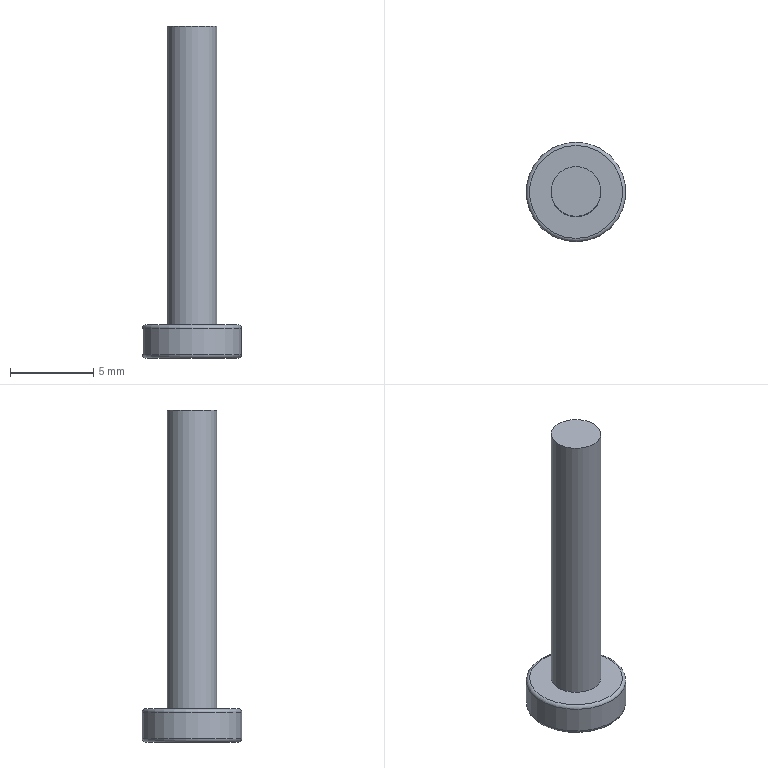Part | STEP file | 1-16.4 | 1 solid | 8 faces | box 6 x 6 x 20 mm | volume 175.087 mm3 | plane 3 | cylinder 2 | torus 2 | cone 1 | commonest cylinder face diameters 3 x1 6 x1
STEP:
#1=CARTESIAN_POINT('',(0.,0.,0.));
#2=DIRECTION('',(0.,0.,1.));
#3=DIRECTION('',(1.,0.,0.));
#4=AXIS2_PLACEMENT_3D('',#1,#2,#3);
#5=CARTESIAN_POINT('',(0.,1.5,0.));
#6=VERTEX_POINT('',#5);
#7=CARTESIAN_POINT('',(0.,0.,0.));
#8=DIRECTION('',(0.,0.,1.));
#9=DIRECTION('',(0.,1.,0.));
#10=AXIS2_PLACEMENT_3D('',#7,#8,#9);
#11=CIRCLE('',#10,1.5);
#12=CARTESIAN_POINT('',(0.,0.,0.));
#13=DIRECTION('',(0.,0.,1.));
#14=DIRECTION('',(0.,1.,0.));
#15=AXIS2_PLACEMENT_3D('',#12,#13,#14);
#16=CYLINDRICAL_SURFACE('',#15,1.5);
#17=CARTESIAN_POINT('',(0.,0.));
#18=DIRECTION('',(1.,0.));
#19=VECTOR('',#18,1.);
#20=LINE('',#17,#19);
#21=(GEOMETRIC_REPRESENTATION_CONTEXT(2)PARAMETRIC_REPRESENTATION_CONTEXT()REPRESENTATION_CONTEXT('',''));
#22=DEFINITIONAL_REPRESENTATION('',(#20),#21);
#23=PCURVE('',#16,#22);
#24=CARTESIAN_POINT('',(0.,-0.8038,0.));
#25=DIRECTION('',(0.,0.,1.));
#26=DIRECTION('',(1.,0.,0.));
#27=AXIS2_PLACEMENT_3D('',#24,#25,#26);
#28=PLANE('',#27);
#29=CARTESIAN_POINT('',(0.,0.8038));
#30=DIRECTION('',(0.,1.));
#31=AXIS2_PLACEMENT_2D('',#29,#30);
#32=CIRCLE('',#31,1.5);
#33=(GEOMETRIC_REPRESENTATION_CONTEXT(2)PARAMETRIC_REPRESENTATION_CONTEXT()REPRESENTATION_CONTEXT('',''));
#34=DEFINITIONAL_REPRESENTATION('',(#32),#33);
#35=PCURVE('',#28,#34);
#36=SURFACE_CURVE('',#11,(#23,#35),.PCURVE_S1.);
#37=EDGE_CURVE('',#6,#6,#36,.T.);
#38=ORIENTED_EDGE('',*,*,#37,.T.);
#39=CARTESIAN_POINT('',(0.,1.5,18.));
#40=VERTEX_POINT('',#39);
#41=CARTESIAN_POINT('',(0.,1.5,0.));
#42=DIRECTION('',(0.,0.,1.));
#43=VECTOR('',#42,1.);
#44=LINE('',#41,#43);
#45=CARTESIAN_POINT('',(6.283,0.));
#46=DIRECTION('',(0.,1.));
#47=VECTOR('',#46,1.);
#48=LINE('',#45,#47);
#49=(GEOMETRIC_REPRESENTATION_CONTEXT(2)PARAMETRIC_REPRESENTATION_CONTEXT()REPRESENTATION_CONTEXT('',''));
#50=DEFINITIONAL_REPRESENTATION('',(#48),#49);
#51=PCURVE('',#16,#50);
#52=CARTESIAN_POINT('',(0.,0.));
#53=DIRECTION('',(0.,1.));
#54=VECTOR('',#53,1.);
#55=LINE('',#52,#54);
#56=(GEOMETRIC_REPRESENTATION_CONTEXT(2)PARAMETRIC_REPRESENTATION_CONTEXT()REPRESENTATION_CONTEXT('',''));
#57=DEFINITIONAL_REPRESENTATION('',(#55),#56);
#58=PCURVE('',#16,#57);
#59=SEAM_CURVE('',#44,(#51,#58),.PCURVE_S1.);
#60=EDGE_CURVE('',#6,#40,#59,.T.);
#61=ORIENTED_EDGE('',*,*,#60,.T.);
#62=CARTESIAN_POINT('',(0.,0.,18.));
#63=DIRECTION('',(0.,0.,1.));
#64=DIRECTION('',(0.,1.,0.));
#65=AXIS2_PLACEMENT_3D('',#62,#63,#64);
#66=CIRCLE('',#65,1.5);
#67=CARTESIAN_POINT('',(0.,18.));
#68=DIRECTION('',(1.,0.));
#69=VECTOR('',#68,1.);
#70=LINE('',#67,#69);
#71=(GEOMETRIC_REPRESENTATION_CONTEXT(2)PARAMETRIC_REPRESENTATION_CONTEXT()REPRESENTATION_CONTEXT('',''));
#72=DEFINITIONAL_REPRESENTATION('',(#70),#71);
#73=PCURVE('',#16,#72);
#74=CARTESIAN_POINT('',(0.,-0.4019,18.));
#75=DIRECTION('',(0.,0.,1.));
#76=DIRECTION('',(1.,0.,0.));
#77=AXIS2_PLACEMENT_3D('',#74,#75,#76);
#78=PLANE('',#77);
#79=CARTESIAN_POINT('',(0.,0.4019));
#80=DIRECTION('',(0.,1.));
#81=AXIS2_PLACEMENT_2D('',#79,#80);
#82=CIRCLE('',#81,1.5);
#83=(GEOMETRIC_REPRESENTATION_CONTEXT(2)PARAMETRIC_REPRESENTATION_CONTEXT()REPRESENTATION_CONTEXT('',''));
#84=DEFINITIONAL_REPRESENTATION('',(#82),#83);
#85=PCURVE('',#78,#84);
#86=SURFACE_CURVE('',#66,(#73,#85),.PCURVE_S1.);
#87=EDGE_CURVE('',#40,#40,#86,.T.);
#88=ORIENTED_EDGE('',*,*,#87,.F.);
#89=ORIENTED_EDGE('',*,*,#60,.F.);
#90=EDGE_LOOP('',(#38,#61,#88,#89));
#91=FACE_BOUND('',#90,.T.);
#92=ADVANCED_FACE('',(#91),#16,.T.);
#93=ORIENTED_EDGE('',*,*,#87,.T.);
#94=EDGE_LOOP('',(#93));
#95=FACE_BOUND('',#94,.T.);
#96=ADVANCED_FACE('',(#95),#78,.T.);
#97=CARTESIAN_POINT('',(0.,3.,-0.2));
#98=VERTEX_POINT('',#97);
#99=CARTESIAN_POINT('',(0.,0.,-0.2));
#100=DIRECTION('',(0.,0.,1.));
#101=DIRECTION('',(0.,1.,0.));
#102=AXIS2_PLACEMENT_3D('',#99,#100,#101);
#103=CIRCLE('',#102,3.);
#104=CARTESIAN_POINT('',(0.,0.,0.));
#105=DIRECTION('',(0.,0.,-1.));
#106=DIRECTION('',(0.,1.,0.));
#107=AXIS2_PLACEMENT_3D('',#104,#105,#106);
#108=CYLINDRICAL_SURFACE('',#107,3.);
#109=CARTESIAN_POINT('',(6.283,0.2));
#110=DIRECTION('',(-1.,0.));
#111=VECTOR('',#110,1.);
#112=LINE('',#109,#111);
#113=(GEOMETRIC_REPRESENTATION_CONTEXT(2)PARAMETRIC_REPRESENTATION_CONTEXT()REPRESENTATION_CONTEXT('',''));
#114=DEFINITIONAL_REPRESENTATION('',(#112),#113);
#115=PCURVE('',#108,#114);
#116=CARTESIAN_POINT('',(0.,0.,-0.2));
#117=DIRECTION('',(0.,0.,-1.));
#118=DIRECTION('',(0.,1.,0.));
#119=AXIS2_PLACEMENT_3D('',#116,#117,#118);
#120=TOROIDAL_SURFACE('',#119,2.8,0.2);
#121=CARTESIAN_POINT('',(6.283,6.283));
#122=DIRECTION('',(-1.,0.));
#123=VECTOR('',#122,1.);
#124=LINE('',#121,#123);
#125=(GEOMETRIC_REPRESENTATION_CONTEXT(2)PARAMETRIC_REPRESENTATION_CONTEXT()REPRESENTATION_CONTEXT('',''));
#126=DEFINITIONAL_REPRESENTATION('',(#124),#125);
#127=PCURVE('',#120,#126);
#128=SURFACE_CURVE('',#103,(#115,#127),.PCURVE_S1.);
#129=EDGE_CURVE('',#98,#98,#128,.T.);
#130=ORIENTED_EDGE('',*,*,#129,.F.);
#131=CARTESIAN_POINT('',(0.,3.,-1.8));
#132=VERTEX_POINT('',#131);
#133=CARTESIAN_POINT('',(0.,3.,-0.2));
#134=DIRECTION('',(0.,0.,-1.));
#135=VECTOR('',#134,1.);
#136=LINE('',#133,#135);
#137=CARTESIAN_POINT('',(6.283,0.2));
#138=DIRECTION('',(0.,1.));
#139=VECTOR('',#138,1.);
#140=LINE('',#137,#139);
#141=(GEOMETRIC_REPRESENTATION_CONTEXT(2)PARAMETRIC_REPRESENTATION_CONTEXT()REPRESENTATION_CONTEXT('',''));
#142=DEFINITIONAL_REPRESENTATION('',(#140),#141);
#143=PCURVE('',#108,#142);
#144=CARTESIAN_POINT('',(0.,0.2));
#145=DIRECTION('',(0.,1.));
#146=VECTOR('',#145,1.);
#147=LINE('',#144,#146);
#148=(GEOMETRIC_REPRESENTATION_CONTEXT(2)PARAMETRIC_REPRESENTATION_CONTEXT()REPRESENTATION_CONTEXT('',''));
#149=DEFINITIONAL_REPRESENTATION('',(#147),#148);
#150=PCURVE('',#108,#149);
#151=SEAM_CURVE('',#136,(#143,#150),.PCURVE_S1.);
#152=EDGE_CURVE('',#98,#132,#151,.T.);
#153=ORIENTED_EDGE('',*,*,#152,.T.);
#154=CARTESIAN_POINT('',(0.,0.,-1.8));
#155=DIRECTION('',(0.,0.,1.));
#156=DIRECTION('',(0.,1.,0.));
#157=AXIS2_PLACEMENT_3D('',#154,#155,#156);
#158=CIRCLE('',#157,3.);
#159=CARTESIAN_POINT('',(6.283,1.8));
#160=DIRECTION('',(-1.,0.));
#161=VECTOR('',#160,1.);
#162=LINE('',#159,#161);
#163=(GEOMETRIC_REPRESENTATION_CONTEXT(2)PARAMETRIC_REPRESENTATION_CONTEXT()REPRESENTATION_CONTEXT('',''));
#164=DEFINITIONAL_REPRESENTATION('',(#162),#163);
#165=PCURVE('',#108,#164);
#166=CARTESIAN_POINT('',(0.,0.,-1.8));
#167=DIRECTION('',(0.,0.,-1.));
#168=DIRECTION('',(0.,1.,0.));
#169=AXIS2_PLACEMENT_3D('',#166,#167,#168);
#170=TOROIDAL_SURFACE('',#169,2.8,0.2);
#171=CARTESIAN_POINT('',(6.283,0.));
#172=DIRECTION('',(-1.,0.));
#173=VECTOR('',#172,1.);
#174=LINE('',#171,#173);
#175=(GEOMETRIC_REPRESENTATION_CONTEXT(2)PARAMETRIC_REPRESENTATION_CONTEXT()REPRESENTATION_CONTEXT('',''));
#176=DEFINITIONAL_REPRESENTATION('',(#174),#175);
#177=PCURVE('',#170,#176);
#178=SURFACE_CURVE('',#158,(#165,#177),.PCURVE_S1.);
#179=EDGE_CURVE('',#132,#132,#178,.T.);
#180=ORIENTED_EDGE('',*,*,#179,.T.);
#181=ORIENTED_EDGE('',*,*,#152,.F.);
#182=EDGE_LOOP('',(#130,#153,#180,#181));
#183=FACE_BOUND('',#182,.T.);
#184=ADVANCED_FACE('',(#183),#108,.T.);
#185=CARTESIAN_POINT('',(0.,2.8,0.));
#186=VERTEX_POINT('',#185);
#187=CARTESIAN_POINT('',(0.,0.,0.));
#188=DIRECTION('',(0.,0.,1.));
#189=DIRECTION('',(0.,1.,0.));
#190=AXIS2_PLACEMENT_3D('',#187,#188,#189);
#191=CIRCLE('',#190,2.8);
#192=CARTESIAN_POINT('',(0.,0.8038));
#193=DIRECTION('',(0.,1.));
#194=AXIS2_PLACEMENT_2D('',#192,#193);
#195=CIRCLE('',#194,2.8);
#196=(GEOMETRIC_REPRESENTATION_CONTEXT(2)PARAMETRIC_REPRESENTATION_CONTEXT()REPRESENTATION_CONTEXT('',''));
#197=DEFINITIONAL_REPRESENTATION('',(#195),#196);
#198=PCURVE('',#28,#197);
#199=CARTESIAN_POINT('',(6.283,4.712));
#200=DIRECTION('',(-1.,0.));
#201=VECTOR('',#200,1.);
#202=LINE('',#199,#201);
#203=(GEOMETRIC_REPRESENTATION_CONTEXT(2)PARAMETRIC_REPRESENTATION_CONTEXT()REPRESENTATION_CONTEXT('',''));
#204=DEFINITIONAL_REPRESENTATION('',(#202),#203);
#205=PCURVE('',#120,#204);
#206=SURFACE_CURVE('',#191,(#198,#205),.PCURVE_S1.);
#207=EDGE_CURVE('',#186,#186,#206,.T.);
#208=ORIENTED_EDGE('',*,*,#207,.T.);
#209=EDGE_LOOP('',(#208));
#210=FACE_BOUND('',#209,.T.);
#211=ORIENTED_EDGE('',*,*,#37,.F.);
#212=EDGE_LOOP('',(#211));
#213=FACE_BOUND('',#212,.T.);
#214=ADVANCED_FACE('',(#210,#213),#28,.T.);
#215=ORIENTED_EDGE('',*,*,#207,.F.);
#216=CARTESIAN_POINT('',(0.,2.8,-0.2));
#217=DIRECTION('',(-1.,0.,0.));
#218=DIRECTION('',(0.,0.,1.));
#219=AXIS2_PLACEMENT_3D('',#216,#217,#218);
#220=CIRCLE('',#219,0.2);
#221=CARTESIAN_POINT('',(6.283,4.712));
#222=DIRECTION('',(0.,1.));
#223=VECTOR('',#222,1.);
#224=LINE('',#221,#223);
#225=(GEOMETRIC_REPRESENTATION_CONTEXT(2)PARAMETRIC_REPRESENTATION_CONTEXT()REPRESENTATION_CONTEXT('',''));
#226=DEFINITIONAL_REPRESENTATION('',(#224),#225);
#227=PCURVE('',#120,#226);
#228=CARTESIAN_POINT('',(0.,4.712));
#229=DIRECTION('',(0.,1.));
#230=VECTOR('',#229,1.);
#231=LINE('',#228,#230);
#232=(GEOMETRIC_REPRESENTATION_CONTEXT(2)PARAMETRIC_REPRESENTATION_CONTEXT()REPRESENTATION_CONTEXT('',''));
#233=DEFINITIONAL_REPRESENTATION('',(#231),#232);
#234=PCURVE('',#120,#233);
#235=SEAM_CURVE('',#220,(#227,#234),.PCURVE_S1.);
#236=EDGE_CURVE('',#186,#98,#235,.T.);
#237=ORIENTED_EDGE('',*,*,#236,.T.);
#238=ORIENTED_EDGE('',*,*,#129,.T.);
#239=ORIENTED_EDGE('',*,*,#236,.F.);
#240=EDGE_LOOP('',(#215,#237,#238,#239));
#241=FACE_BOUND('',#240,.T.);
#242=ADVANCED_FACE('',(#241),#120,.T.);
#243=CARTESIAN_POINT('',(0.,2.8,-2.));
#244=VERTEX_POINT('',#243);
#245=CARTESIAN_POINT('',(0.,2.8,-1.8));
#246=DIRECTION('',(1.,0.,0.));
#247=DIRECTION('',(0.,0.,-1.));
#248=AXIS2_PLACEMENT_3D('',#245,#246,#247);
#249=CIRCLE('',#248,0.2);
#250=CARTESIAN_POINT('',(0.,1.571));
#251=DIRECTION('',(0.,-1.));
#252=VECTOR('',#251,1.);
#253=LINE('',#250,#252);
#254=(GEOMETRIC_REPRESENTATION_CONTEXT(2)PARAMETRIC_REPRESENTATION_CONTEXT()REPRESENTATION_CONTEXT('',''));
#255=DEFINITIONAL_REPRESENTATION('',(#253),#254);
#256=PCURVE('',#170,#255);
#257=CARTESIAN_POINT('',(6.283,1.571));
#258=DIRECTION('',(0.,-1.));
#259=VECTOR('',#258,1.);
#260=LINE('',#257,#259);
#261=(GEOMETRIC_REPRESENTATION_CONTEXT(2)PARAMETRIC_REPRESENTATION_CONTEXT()REPRESENTATION_CONTEXT('',''));
#262=DEFINITIONAL_REPRESENTATION('',(#260),#261);
#263=PCURVE('',#170,#262);
#264=SEAM_CURVE('',#249,(#256,#263),.PCURVE_S1.);
#265=EDGE_CURVE('',#244,#132,#264,.T.);
#266=ORIENTED_EDGE('',*,*,#265,.T.);
#267=ORIENTED_EDGE('',*,*,#179,.F.);
#268=ORIENTED_EDGE('',*,*,#265,.F.);
#269=CARTESIAN_POINT('',(0.,0.,-2.));
#270=DIRECTION('',(0.,0.,1.));
#271=DIRECTION('',(0.,1.,0.));
#272=AXIS2_PLACEMENT_3D('',#269,#270,#271);
#273=CIRCLE('',#272,2.8);
#274=CARTESIAN_POINT('',(6.283,1.571));
#275=DIRECTION('',(-1.,0.));
#276=VECTOR('',#275,1.);
#277=LINE('',#274,#276);
#278=(GEOMETRIC_REPRESENTATION_CONTEXT(2)PARAMETRIC_REPRESENTATION_CONTEXT()REPRESENTATION_CONTEXT('',''));
#279=DEFINITIONAL_REPRESENTATION('',(#277),#278);
#280=PCURVE('',#170,#279);
#281=CARTESIAN_POINT('',(0.,-0.8038,-2.));
#282=DIRECTION('',(0.,0.,1.));
#283=DIRECTION('',(1.,0.,0.));
#284=AXIS2_PLACEMENT_3D('',#281,#282,#283);
#285=PLANE('',#284);
#286=CARTESIAN_POINT('',(0.,0.8038));
#287=DIRECTION('',(0.,1.));
#288=AXIS2_PLACEMENT_2D('',#286,#287);
#289=CIRCLE('',#288,2.8);
#290=(GEOMETRIC_REPRESENTATION_CONTEXT(2)PARAMETRIC_REPRESENTATION_CONTEXT()REPRESENTATION_CONTEXT('',''));
#291=DEFINITIONAL_REPRESENTATION('',(#289),#290);
#292=PCURVE('',#285,#291);
#293=SURFACE_CURVE('',#273,(#280,#292),.PCURVE_S1.);
#294=EDGE_CURVE('',#244,#244,#293,.T.);
#295=ORIENTED_EDGE('',*,*,#294,.T.);
#296=EDGE_LOOP('',(#266,#267,#268,#295));
#297=FACE_BOUND('',#296,.T.);
#298=ADVANCED_FACE('',(#297),#170,.T.);
#299=ORIENTED_EDGE('',*,*,#294,.T.);
#300=EDGE_LOOP('',(#299));
#301=FACE_BOUND('',#300,.F.);
#302=CARTESIAN_POINT('',(0.,2.,-2.));
#303=VERTEX_POINT('',#302);
#304=CARTESIAN_POINT('',(0.,0.,-2.));
#305=DIRECTION('',(0.,0.,-1.));
#306=DIRECTION('',(0.,1.,0.));
#307=AXIS2_PLACEMENT_3D('',#304,#305,#306);
#308=CIRCLE('',#307,2.);
#309=CARTESIAN_POINT('',(0.,2.804));
#310=CARTESIAN_POINT('',(3.464,2.804));
#311=CARTESIAN_POINT('',(1.732,-0.1962));
#312=CARTESIAN_POINT('',(0.,-3.196));
#313=CARTESIAN_POINT('',(-1.732,-0.1962));
#314=CARTESIAN_POINT('',(-3.464,2.804));
#315=CARTESIAN_POINT('',(0.,2.804));
#316=(BOUNDED_CURVE()B_SPLINE_CURVE(2,(#309,#310,#311,#312,#313,#314,#315),.UNSPECIFIED.,.T.,.F.)B_SPLINE_CURVE_WITH_KNOTS((1,2,2,2,2,1),(-2.094,0.,2.094,4.189,6.283,8.378),.UNSPECIFIED.)CURVE()GEOMETRIC_REPRESENTATION_ITEM()RATIONAL_B_SPLINE_CURVE((1.,0.5,1.,0.5,1.,0.5,1.))REPRESENTATION_ITEM(''));
#317=(GEOMETRIC_REPRESENTATION_CONTEXT(2)PARAMETRIC_REPRESENTATION_CONTEXT()REPRESENTATION_CONTEXT('',''));
#318=DEFINITIONAL_REPRESENTATION('',(#316),#317);
#319=PCURVE('',#285,#318);
#320=CARTESIAN_POINT('',(0.,0.,0.));
#321=DIRECTION('',(0.,0.,-1.));
#322=DIRECTION('',(0.,1.,0.));
#323=AXIS2_PLACEMENT_3D('',#320,#321,#322);
#324=CONICAL_SURFACE('',#323,0.,0.7854);
#325=CARTESIAN_POINT('',(0.,2.));
#326=DIRECTION('',(1.,0.));
#327=VECTOR('',#326,1.);
#328=LINE('',#325,#327);
#329=(GEOMETRIC_REPRESENTATION_CONTEXT(2)PARAMETRIC_REPRESENTATION_CONTEXT()REPRESENTATION_CONTEXT('',''));
#330=DEFINITIONAL_REPRESENTATION('',(#328),#329);
#331=PCURVE('',#324,#330);
#332=SURFACE_CURVE('',#308,(#319,#331),.PCURVE_S1.);
#333=EDGE_CURVE('',#303,#303,#332,.T.);
#334=ORIENTED_EDGE('',*,*,#333,.T.);
#335=EDGE_LOOP('',(#334));
#336=FACE_BOUND('',#335,.F.);
#337=ADVANCED_FACE('',(#301,#336),#285,.F.);
#338=CARTESIAN_POINT('',(0.,0.,0.));
#339=VERTEX_POINT('',#338);
#340=CARTESIAN_POINT('',(0.,2.,-2.));
#341=DIRECTION('',(0.,-0.7071,0.7071));
#342=VECTOR('',#341,1.);
#343=LINE('',#340,#342);
#344=CARTESIAN_POINT('',(0.,2.));
#345=CARTESIAN_POINT('',(0.,1.97));
#346=CARTESIAN_POINT('',(0.,1.909));
#347=CARTESIAN_POINT('',(0.,1.818));
#348=CARTESIAN_POINT('',(0.,1.727));
#349=CARTESIAN_POINT('',(0.,1.636));
#350=CARTESIAN_POINT('',(0.,1.545));
#351=CARTESIAN_POINT('',(0.,1.455));
#352=CARTESIAN_POINT('',(0.,1.364));
#353=CARTESIAN_POINT('',(0.,1.273));
#354=CARTESIAN_POINT('',(0.,1.182));
#355=CARTESIAN_POINT('',(0.,1.091));
#356=CARTESIAN_POINT('',(0.,1.));
#357=CARTESIAN_POINT('',(0.,0.9091));
#358=CARTESIAN_POINT('',(0.,0.8182));
#359=CARTESIAN_POINT('',(0.,0.7273));
#360=CARTESIAN_POINT('',(0.,0.6364));
#361=CARTESIAN_POINT('',(0.,0.5455));
#362=CARTESIAN_POINT('',(0.,0.4545));
#363=CARTESIAN_POINT('',(0.,0.3636));
#364=CARTESIAN_POINT('',(0.,0.2727));
#365=CARTESIAN_POINT('',(0.,0.1818));
#366=CARTESIAN_POINT('',(0.,0.09091));
#367=CARTESIAN_POINT('',(0.,0.0303));
#368=CARTESIAN_POINT('',(0.,0.));
#369=B_SPLINE_CURVE_WITH_KNOTS('',3,(#344,#345,#346,#347,#348,#349,#350,#351,#352,#353,#354,#355,#356,#357,#358,#359,#360,#361,#362,#363,#364,#365,#366,#367,#368),.UNSPECIFIED.,.F.,.F.,(4,1,1,1,1,1,1,1,1,1,1,1,1,1,1,1,1,1,1,1,1,1,4),(0.,0.1286,0.2571,0.3857,0.5143,0.6428,0.7714,0.9,1.029,1.157,1.286,1.414,1.543,1.671,1.8,1.928,2.057,2.186,2.314,2.443,2.571,2.7,2.828),.QUASI_UNIFORM_KNOTS.);
#370=(GEOMETRIC_REPRESENTATION_CONTEXT(2)PARAMETRIC_REPRESENTATION_CONTEXT()REPRESENTATION_CONTEXT('',''));
#371=DEFINITIONAL_REPRESENTATION('',(#369),#370);
#372=PCURVE('',#324,#371);
#373=CARTESIAN_POINT('',(6.283,2.));
#374=CARTESIAN_POINT('',(6.283,1.97));
#375=CARTESIAN_POINT('',(6.283,1.909));
#376=CARTESIAN_POINT('',(6.283,1.818));
#377=CARTESIAN_POINT('',(6.283,1.727));
#378=CARTESIAN_POINT('',(6.283,1.636));
#379=CARTESIAN_POINT('',(6.283,1.545));
#380=CARTESIAN_POINT('',(6.283,1.455));
#381=CARTESIAN_POINT('',(6.283,1.364));
#382=CARTESIAN_POINT('',(6.283,1.273));
#383=CARTESIAN_POINT('',(6.283,1.182));
#384=CARTESIAN_POINT('',(6.283,1.091));
#385=CARTESIAN_POINT('',(6.283,1.));
#386=CARTESIAN_POINT('',(6.283,0.9091));
#387=CARTESIAN_POINT('',(6.283,0.8182));
#388=CARTESIAN_POINT('',(6.283,0.7273));
#389=CARTESIAN_POINT('',(6.283,0.6364));
#390=CARTESIAN_POINT('',(6.283,0.5455));
#391=CARTESIAN_POINT('',(6.283,0.4545));
#392=CARTESIAN_POINT('',(6.283,0.3636));
#393=CARTESIAN_POINT('',(6.283,0.2727));
#394=CARTESIAN_POINT('',(6.283,0.1818));
#395=CARTESIAN_POINT('',(6.283,0.09091));
#396=CARTESIAN_POINT('',(6.283,0.0303));
#397=CARTESIAN_POINT('',(6.283,0.));
#398=B_SPLINE_CURVE_WITH_KNOTS('',3,(#373,#374,#375,#376,#377,#378,#379,#380,#381,#382,#383,#384,#385,#386,#387,#388,#389,#390,#391,#392,#393,#394,#395,#396,#397),.UNSPECIFIED.,.F.,.F.,(4,1,1,1,1,1,1,1,1,1,1,1,1,1,1,1,1,1,1,1,1,1,4),(0.,0.1286,0.2571,0.3857,0.5143,0.6428,0.7714,0.9,1.029,1.157,1.286,1.414,1.543,1.671,1.8,1.928,2.057,2.186,2.314,2.443,2.571,2.7,2.828),.QUASI_UNIFORM_KNOTS.);
#399=(GEOMETRIC_REPRESENTATION_CONTEXT(2)PARAMETRIC_REPRESENTATION_CONTEXT()REPRESENTATION_CONTEXT('',''));
#400=DEFINITIONAL_REPRESENTATION('',(#398),#399);
#401=PCURVE('',#324,#400);
#402=SEAM_CURVE('',#343,(#372,#401),.PCURVE_S1.);
#403=EDGE_CURVE('',#303,#339,#402,.T.);
#404=ORIENTED_EDGE('',*,*,#403,.T.);
#405=ORIENTED_EDGE('',*,*,#403,.F.);
#406=ORIENTED_EDGE('',*,*,#333,.F.);
#407=EDGE_LOOP('',(#404,#405,#406));
#408=FACE_BOUND('',#407,.F.);
#409=ADVANCED_FACE('',(#408),#324,.F.);
#410=CLOSED_SHELL('',(#92,#96,#184,#214,#242,#298,#337,#409));
#411=MANIFOLD_SOLID_BREP('',#410);
#412=(LENGTH_UNIT()NAMED_UNIT(*)SI_UNIT(.MILLI.,.METRE.));
#413=UNCERTAINTY_MEASURE_WITH_UNIT(LENGTH_MEASURE(0.0000001),#412,'','');
#414=(NAMED_UNIT(*)PLANE_ANGLE_UNIT()SI_UNIT($,.RADIAN.));
#415=(NAMED_UNIT(*)SI_UNIT($,.STERADIAN.)SOLID_ANGLE_UNIT());
#416=(GEOMETRIC_REPRESENTATION_CONTEXT(3)GLOBAL_UNCERTAINTY_ASSIGNED_CONTEXT((#413))GLOBAL_UNIT_ASSIGNED_CONTEXT((#412,#414,#415))REPRESENTATION_CONTEXT('',''));
#417=ADVANCED_BREP_SHAPE_REPRESENTATION('',(#4,#411),#416);